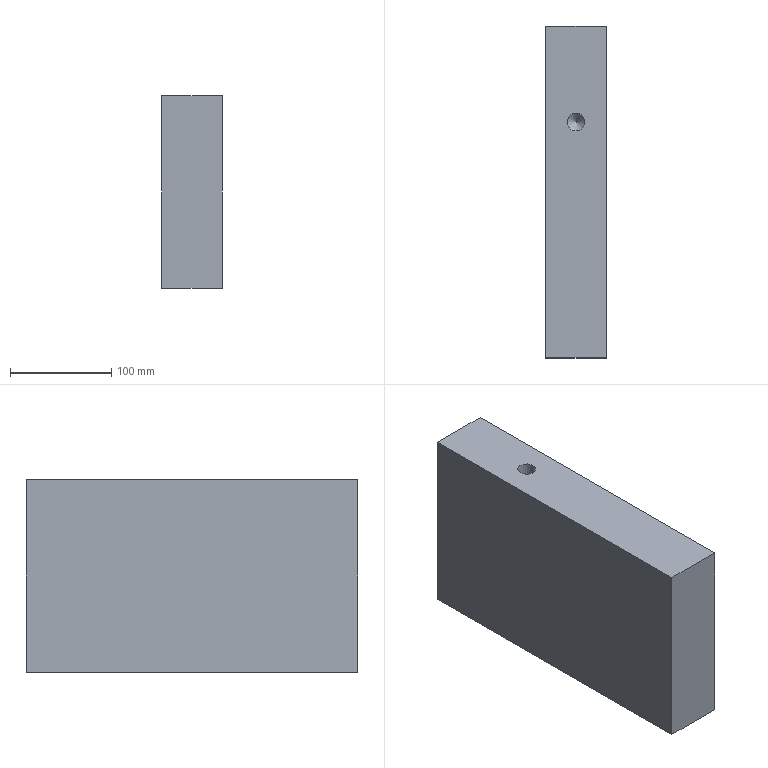Part | STEP file | lll_id4114_x_t | 1 solid | 12 faces | box 60 x 328 x 190 mm | volume 3707305 mm3 | plane 6 | cylinder 3 | cone 3 | commonest cylinder face diameters 17.506 x3
STEP:
#1=CARTESIAN_POINT('',(3516.188,365.,-370.));
#2=VERTEX_POINT('',#1);
#3=CARTESIAN_POINT('',(3507.435,365.,-370.));
#4=DIRECTION('',(0.,0.,1.));
#5=DIRECTION('',(1.,0.,0.));
#6=AXIS2_PLACEMENT_3D('',#3,#4,#5);
#7=CIRCLE('',#6,8.753);
#8=EDGE_CURVE('',#2,#2,#7,.T.);
#9=ORIENTED_EDGE('',*,*,#8,.T.);
#10=EDGE_LOOP('',(#9));
#11=FACE_BOUND('',#10,.T.);
#12=CARTESIAN_POINT('',(3477.435,272.,-370.));
#13=VERTEX_POINT('',#12);
#14=CARTESIAN_POINT('',(3537.435,272.,-370.));
#15=VERTEX_POINT('',#14);
#16=CARTESIAN_POINT('',(5723.751,272.,-370.));
#17=DIRECTION('',(1.,0.,0.));
#18=VECTOR('',#17,1.);
#19=LINE('',#16,#18);
#20=EDGE_CURVE('',#13,#15,#19,.T.);
#21=ORIENTED_EDGE('',*,*,#20,.F.);
#22=CARTESIAN_POINT('',(3477.435,600.,-370.));
#23=VERTEX_POINT('',#22);
#24=CARTESIAN_POINT('',(3477.435,-1.,-370.));
#25=DIRECTION('',(0.,1.,0.));
#26=VECTOR('',#25,1.);
#27=LINE('',#24,#26);
#28=EDGE_CURVE('',#13,#23,#27,.T.);
#29=ORIENTED_EDGE('',*,*,#28,.T.);
#30=CARTESIAN_POINT('',(3537.435,600.,-370.));
#31=VERTEX_POINT('',#30);
#32=CARTESIAN_POINT('',(3537.435,600.,-370.));
#33=DIRECTION('',(-1.,0.,0.));
#34=VECTOR('',#33,1.);
#35=LINE('',#32,#34);
#36=EDGE_CURVE('',#31,#23,#35,.T.);
#37=ORIENTED_EDGE('',*,*,#36,.F.);
#38=CARTESIAN_POINT('',(3537.435,-600.,-370.));
#39=DIRECTION('',(0.,1.,0.));
#40=VECTOR('',#39,1.);
#41=LINE('',#38,#40);
#42=EDGE_CURVE('',#15,#31,#41,.T.);
#43=ORIENTED_EDGE('',*,*,#42,.F.);
#44=EDGE_LOOP('',(#21,#29,#37,#43));
#45=FACE_BOUND('',#44,.T.);
#46=CARTESIAN_POINT('',(3516.188,550.,-370.));
#47=VERTEX_POINT('',#46);
#48=CARTESIAN_POINT('',(3507.435,550.,-370.));
#49=DIRECTION('',(0.,0.,1.));
#50=DIRECTION('',(1.,0.,0.));
#51=AXIS2_PLACEMENT_3D('',#48,#49,#50);
#52=CIRCLE('',#51,8.753);
#53=EDGE_CURVE('',#47,#47,#52,.T.);
#54=ORIENTED_EDGE('',*,*,#53,.T.);
#55=EDGE_LOOP('',(#54));
#56=FACE_BOUND('',#55,.T.);
#57=CARTESIAN_POINT('',(5723.751,-1.,-370.));
#58=DIRECTION('',(0.,0.,-1.));
#59=DIRECTION('',(-1.,0.,0.));
#60=AXIS2_PLACEMENT_3D('',#57,#58,#59);
#61=PLANE('',#60);
#62=ADVANCED_FACE('',(#11,#45,#56),#61,.T.);
#63=CARTESIAN_POINT('',(3537.435,272.,-180.));
#64=VERTEX_POINT('',#63);
#65=CARTESIAN_POINT('',(3537.435,600.,-180.));
#66=VERTEX_POINT('',#65);
#67=CARTESIAN_POINT('',(3537.435,-1.,-180.));
#68=DIRECTION('',(0.,1.,0.));
#69=VECTOR('',#68,1.);
#70=LINE('',#67,#69);
#71=EDGE_CURVE('',#64,#66,#70,.T.);
#72=ORIENTED_EDGE('',*,*,#71,.F.);
#73=CARTESIAN_POINT('',(3537.435,272.,-182.5));
#74=DIRECTION('',(0.,0.,1.));
#75=VECTOR('',#74,1.);
#76=LINE('',#73,#75);
#77=EDGE_CURVE('',#15,#64,#76,.T.);
#78=ORIENTED_EDGE('',*,*,#77,.F.);
#79=ORIENTED_EDGE('',*,*,#42,.T.);
#80=CARTESIAN_POINT('',(3537.435,600.,-182.5));
#81=DIRECTION('',(0.,0.,-1.));
#82=VECTOR('',#81,1.);
#83=LINE('',#80,#82);
#84=EDGE_CURVE('',#66,#31,#83,.T.);
#85=ORIENTED_EDGE('',*,*,#84,.F.);
#86=EDGE_LOOP('',(#72,#78,#79,#85));
#87=FACE_OUTER_BOUND('',#86,.T.);
#88=CARTESIAN_POINT('',(3537.435,-600.,-182.5));
#89=DIRECTION('',(1.,0.,0.));
#90=DIRECTION('',(0.,0.,-1.));
#91=AXIS2_PLACEMENT_3D('',#88,#89,#90);
#92=PLANE('',#91);
#93=ADVANCED_FACE('',(#87),#92,.T.);
#94=CARTESIAN_POINT('',(3477.435,272.,-180.));
#95=VERTEX_POINT('',#94);
#96=CARTESIAN_POINT('',(3477.435,272.,-251.25));
#97=DIRECTION('',(0.,0.,1.));
#98=VECTOR('',#97,1.);
#99=LINE('',#96,#98);
#100=EDGE_CURVE('',#13,#95,#99,.T.);
#101=ORIENTED_EDGE('',*,*,#100,.T.);
#102=CARTESIAN_POINT('',(3477.435,600.,-180.));
#103=VERTEX_POINT('',#102);
#104=CARTESIAN_POINT('',(3477.435,0.,-180.));
#105=DIRECTION('',(0.,-1.,0.));
#106=VECTOR('',#105,1.);
#107=LINE('',#104,#106);
#108=EDGE_CURVE('',#103,#95,#107,.T.);
#109=ORIENTED_EDGE('',*,*,#108,.F.);
#110=CARTESIAN_POINT('',(3477.435,600.,-182.5));
#111=DIRECTION('',(0.,0.,-1.));
#112=VECTOR('',#111,1.);
#113=LINE('',#110,#112);
#114=EDGE_CURVE('',#103,#23,#113,.T.);
#115=ORIENTED_EDGE('',*,*,#114,.T.);
#116=ORIENTED_EDGE('',*,*,#28,.F.);
#117=EDGE_LOOP('',(#101,#109,#115,#116));
#118=FACE_OUTER_BOUND('',#117,.T.);
#119=CARTESIAN_POINT('',(3477.435,0.,-251.25));
#120=DIRECTION('',(1.,0.,0.));
#121=DIRECTION('',(0.,0.,-1.));
#122=AXIS2_PLACEMENT_3D('',#119,#120,#121);
#123=PLANE('',#122);
#124=ADVANCED_FACE('',(#118),#123,.F.);
#125=CARTESIAN_POINT('',(3498.682,505.,-180.));
#126=VERTEX_POINT('',#125);
#127=CARTESIAN_POINT('',(3507.435,505.,-180.));
#128=DIRECTION('',(0.,0.,-1.));
#129=DIRECTION('',(-1.,0.,0.));
#130=AXIS2_PLACEMENT_3D('',#127,#128,#129);
#131=CIRCLE('',#130,8.753);
#132=EDGE_CURVE('',#126,#126,#131,.T.);
#133=ORIENTED_EDGE('',*,*,#132,.T.);
#134=EDGE_LOOP('',(#133));
#135=FACE_BOUND('',#134,.T.);
#136=CARTESIAN_POINT('',(3987.723,272.,-180.));
#137=DIRECTION('',(-1.,0.,0.));
#138=VECTOR('',#137,1.);
#139=LINE('',#136,#138);
#140=EDGE_CURVE('',#64,#95,#139,.T.);
#141=ORIENTED_EDGE('',*,*,#140,.F.);
#142=ORIENTED_EDGE('',*,*,#71,.T.);
#143=CARTESIAN_POINT('',(5723.751,600.,-180.));
#144=DIRECTION('',(-1.,0.,0.));
#145=VECTOR('',#144,1.);
#146=LINE('',#143,#145);
#147=EDGE_CURVE('',#66,#103,#146,.T.);
#148=ORIENTED_EDGE('',*,*,#147,.T.);
#149=ORIENTED_EDGE('',*,*,#108,.T.);
#150=EDGE_LOOP('',(#141,#142,#148,#149));
#151=FACE_BOUND('',#150,.T.);
#152=CARTESIAN_POINT('',(5723.751,-1.,-180.));
#153=DIRECTION('',(0.,0.,-1.));
#154=DIRECTION('',(-1.,0.,0.));
#155=AXIS2_PLACEMENT_3D('',#152,#153,#154);
#156=PLANE('',#155);
#157=ADVANCED_FACE('',(#135,#151),#156,.F.);
#158=ORIENTED_EDGE('',*,*,#114,.F.);
#159=ORIENTED_EDGE('',*,*,#147,.F.);
#160=ORIENTED_EDGE('',*,*,#84,.T.);
#161=ORIENTED_EDGE('',*,*,#36,.T.);
#162=EDGE_LOOP('',(#158,#159,#160,#161));
#163=FACE_OUTER_BOUND('',#162,.T.);
#164=CARTESIAN_POINT('',(3537.435,600.,-182.5));
#165=DIRECTION('',(0.,1.,0.));
#166=DIRECTION('',(0.,0.,-1.));
#167=AXIS2_PLACEMENT_3D('',#164,#165,#166);
#168=PLANE('',#167);
#169=ADVANCED_FACE('',(#163),#168,.T.);
#170=ORIENTED_EDGE('',*,*,#20,.T.);
#171=ORIENTED_EDGE('',*,*,#77,.T.);
#172=ORIENTED_EDGE('',*,*,#140,.T.);
#173=ORIENTED_EDGE('',*,*,#100,.F.);
#174=EDGE_LOOP('',(#170,#171,#172,#173));
#175=FACE_OUTER_BOUND('',#174,.T.);
#176=CARTESIAN_POINT('',(3987.723,272.,-141.707));
#177=DIRECTION('',(0.,1.,0.));
#178=DIRECTION('',(-0.9063,0.,-0.4226));
#179=AXIS2_PLACEMENT_3D('',#176,#177,#178);
#180=PLANE('',#179);
#181=ADVANCED_FACE('',(#175),#180,.F.);
#182=CARTESIAN_POINT('',(3498.682,505.,-221.253));
#183=VERTEX_POINT('',#182);
#184=CARTESIAN_POINT('',(3507.435,505.,-221.253));
#185=DIRECTION('',(0.,0.,-1.));
#186=DIRECTION('',(-1.,0.,0.));
#187=AXIS2_PLACEMENT_3D('',#184,#185,#186);
#188=CIRCLE('',#187,8.753);
#189=EDGE_CURVE('',#183,#183,#188,.T.);
#190=ORIENTED_EDGE('',*,*,#189,.T.);
#191=EDGE_LOOP('',(#190));
#192=FACE_BOUND('',#191,.T.);
#193=ORIENTED_EDGE('',*,*,#132,.F.);
#194=EDGE_LOOP('',(#193));
#195=FACE_BOUND('',#194,.T.);
#196=CARTESIAN_POINT('',(3507.435,505.,-180.));
#197=DIRECTION('',(0.,0.,-1.));
#198=DIRECTION('',(1.,0.,0.));
#199=AXIS2_PLACEMENT_3D('',#196,#197,#198);
#200=CYLINDRICAL_SURFACE('',#199,8.753);
#201=ADVANCED_FACE('',(#192,#195),#200,.F.);
#202=CARTESIAN_POINT('',(3507.435,505.,-230.006));
#203=VERTEX_POINT('',#202);
#204=VERTEX_LOOP('',#203);
#205=FACE_BOUND('',#204,.T.);
#206=ORIENTED_EDGE('',*,*,#189,.F.);
#207=EDGE_LOOP('',(#206));
#208=FACE_BOUND('',#207,.T.);
#209=CARTESIAN_POINT('',(3507.435,505.,-221.253));
#210=DIRECTION('',(0.,0.,1.));
#211=DIRECTION('',(-1.,0.,0.));
#212=AXIS2_PLACEMENT_3D('',#209,#210,#211);
#213=CONICAL_SURFACE('',#212,8.753,45.);
#214=ADVANCED_FACE('',(#205,#208),#213,.F.);
#215=CARTESIAN_POINT('',(3516.188,365.,-328.747));
#216=VERTEX_POINT('',#215);
#217=CARTESIAN_POINT('',(3507.435,365.,-328.747));
#218=DIRECTION('',(0.,0.,1.));
#219=DIRECTION('',(1.,0.,0.));
#220=AXIS2_PLACEMENT_3D('',#217,#218,#219);
#221=CIRCLE('',#220,8.753);
#222=EDGE_CURVE('',#216,#216,#221,.T.);
#223=ORIENTED_EDGE('',*,*,#222,.T.);
#224=EDGE_LOOP('',(#223));
#225=FACE_BOUND('',#224,.T.);
#226=ORIENTED_EDGE('',*,*,#8,.F.);
#227=EDGE_LOOP('',(#226));
#228=FACE_BOUND('',#227,.T.);
#229=CARTESIAN_POINT('',(3507.435,365.,-370.));
#230=DIRECTION('',(0.,0.,1.));
#231=DIRECTION('',(-1.,0.,0.));
#232=AXIS2_PLACEMENT_3D('',#229,#230,#231);
#233=CYLINDRICAL_SURFACE('',#232,8.753);
#234=ADVANCED_FACE('',(#225,#228),#233,.F.);
#235=CARTESIAN_POINT('',(3507.435,365.,-319.994));
#236=VERTEX_POINT('',#235);
#237=VERTEX_LOOP('',#236);
#238=FACE_BOUND('',#237,.T.);
#239=ORIENTED_EDGE('',*,*,#222,.F.);
#240=EDGE_LOOP('',(#239));
#241=FACE_BOUND('',#240,.T.);
#242=CARTESIAN_POINT('',(3507.435,365.,-328.747));
#243=DIRECTION('',(0.,0.,-1.));
#244=DIRECTION('',(1.,0.,0.));
#245=AXIS2_PLACEMENT_3D('',#242,#243,#244);
#246=CONICAL_SURFACE('',#245,8.753,45.);
#247=ADVANCED_FACE('',(#238,#241),#246,.F.);
#248=CARTESIAN_POINT('',(3516.188,550.,-328.747));
#249=VERTEX_POINT('',#248);
#250=CARTESIAN_POINT('',(3507.435,550.,-328.747));
#251=DIRECTION('',(0.,0.,1.));
#252=DIRECTION('',(1.,0.,0.));
#253=AXIS2_PLACEMENT_3D('',#250,#251,#252);
#254=CIRCLE('',#253,8.753);
#255=EDGE_CURVE('',#249,#249,#254,.T.);
#256=ORIENTED_EDGE('',*,*,#255,.T.);
#257=EDGE_LOOP('',(#256));
#258=FACE_BOUND('',#257,.T.);
#259=ORIENTED_EDGE('',*,*,#53,.F.);
#260=EDGE_LOOP('',(#259));
#261=FACE_BOUND('',#260,.T.);
#262=CARTESIAN_POINT('',(3507.435,550.,-370.));
#263=DIRECTION('',(0.,0.,1.));
#264=DIRECTION('',(-1.,0.,0.));
#265=AXIS2_PLACEMENT_3D('',#262,#263,#264);
#266=CYLINDRICAL_SURFACE('',#265,8.753);
#267=ADVANCED_FACE('',(#258,#261),#266,.F.);
#268=CARTESIAN_POINT('',(3507.435,550.,-319.994));
#269=VERTEX_POINT('',#268);
#270=VERTEX_LOOP('',#269);
#271=FACE_BOUND('',#270,.T.);
#272=ORIENTED_EDGE('',*,*,#255,.F.);
#273=EDGE_LOOP('',(#272));
#274=FACE_BOUND('',#273,.T.);
#275=CARTESIAN_POINT('',(3507.435,550.,-328.747));
#276=DIRECTION('',(0.,0.,-1.));
#277=DIRECTION('',(1.,0.,0.));
#278=AXIS2_PLACEMENT_3D('',#275,#276,#277);
#279=CONICAL_SURFACE('',#278,8.753,45.);
#280=ADVANCED_FACE('',(#271,#274),#279,.F.);
#281=CLOSED_SHELL('',(#62,#93,#124,#157,#169,#181,#201,#214,#234,#247,#267,#280));
#282=MANIFOLD_SOLID_BREP('',#281);
#283=(LENGTH_UNIT()NAMED_UNIT(*)SI_UNIT(.MILLI.,.METRE.));
#284=UNCERTAINTY_MEASURE_WITH_UNIT(LENGTH_MEASURE(0.00002),#283,'','');
#285=(NAMED_UNIT(*)PLANE_ANGLE_UNIT()SI_UNIT($,.RADIAN.));
#286=PLANE_ANGLE_MEASURE_WITH_UNIT(PLANE_ANGLE_MEASURE(0.01745),#285);
#287=DIMENSIONAL_EXPONENTS(0.,0.,0.,0.,0.,0.,0.);
#288=(CONVERSION_BASED_UNIT('DEGREE',#286)NAMED_UNIT(#287)PLANE_ANGLE_UNIT());
#289=(NAMED_UNIT(*)SI_UNIT($,.STERADIAN.)SOLID_ANGLE_UNIT());
#290=(GEOMETRIC_REPRESENTATION_CONTEXT(3)GLOBAL_UNCERTAINTY_ASSIGNED_CONTEXT((#284))GLOBAL_UNIT_ASSIGNED_CONTEXT((#283,#288,#289))REPRESENTATION_CONTEXT('',''));
#291=ADVANCED_BREP_SHAPE_REPRESENTATION('',(#282),#290);